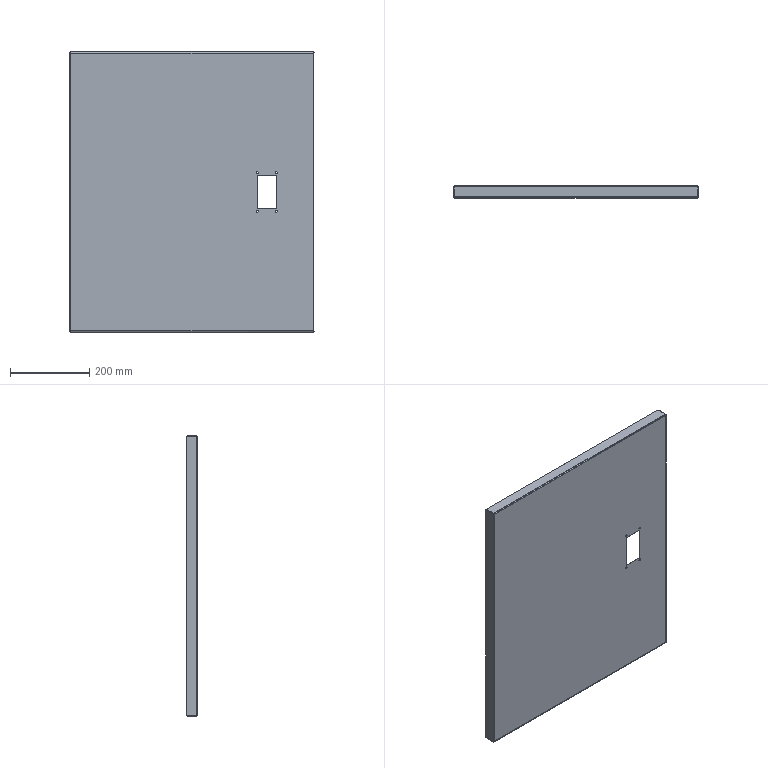Part | STEP file | SOLID | 1 solid | 110 faces | box 615 x 30 x 705 mm | volume 627775 mm3 | plane 58 | spline 32 | cylinder 20 | commonest cylinder face diameters 3 x8 5.4 x8 4.5 x4